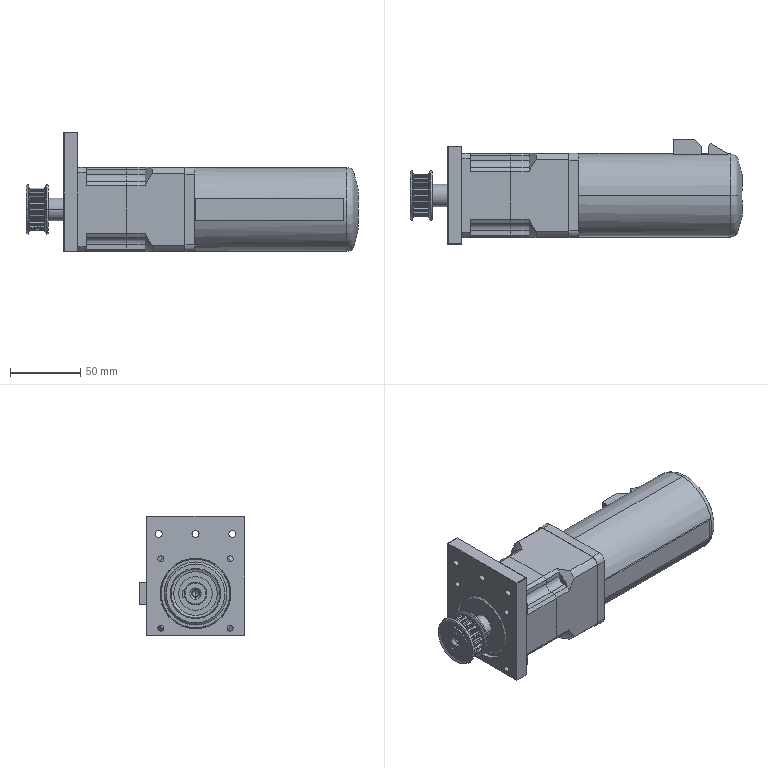Part | NX | 5 solids | 515 faces | box 237 x 75 x 85 mm | volume 624353 mm3 | cylinder 323 | plane 122 | cone 60 | torus 10 | commonest cylinder face diameters 6.55 x44 0.5 x43 1.1 x42 30.87 x42 27.33 x21 69 x16